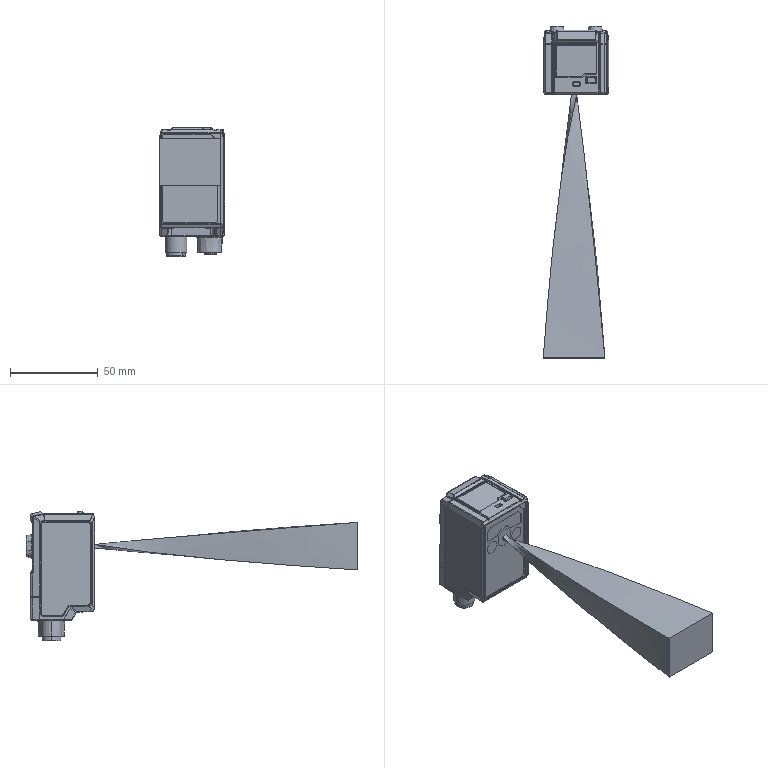Part | STEP file | sr-x100^Scanner moving assembly | 1 solid | 2023 faces | box 37.2 x 188.7 x 73.89 mm | volume 134678 mm3 | cylinder 655 | plane 621 | spline 566 | cone 79 | torus 67 | sphere 35 | commonest cylinder face diameters 0.2 x170 0.6 x144 0.4 x115 1 x63 1.8 x38 2 x28